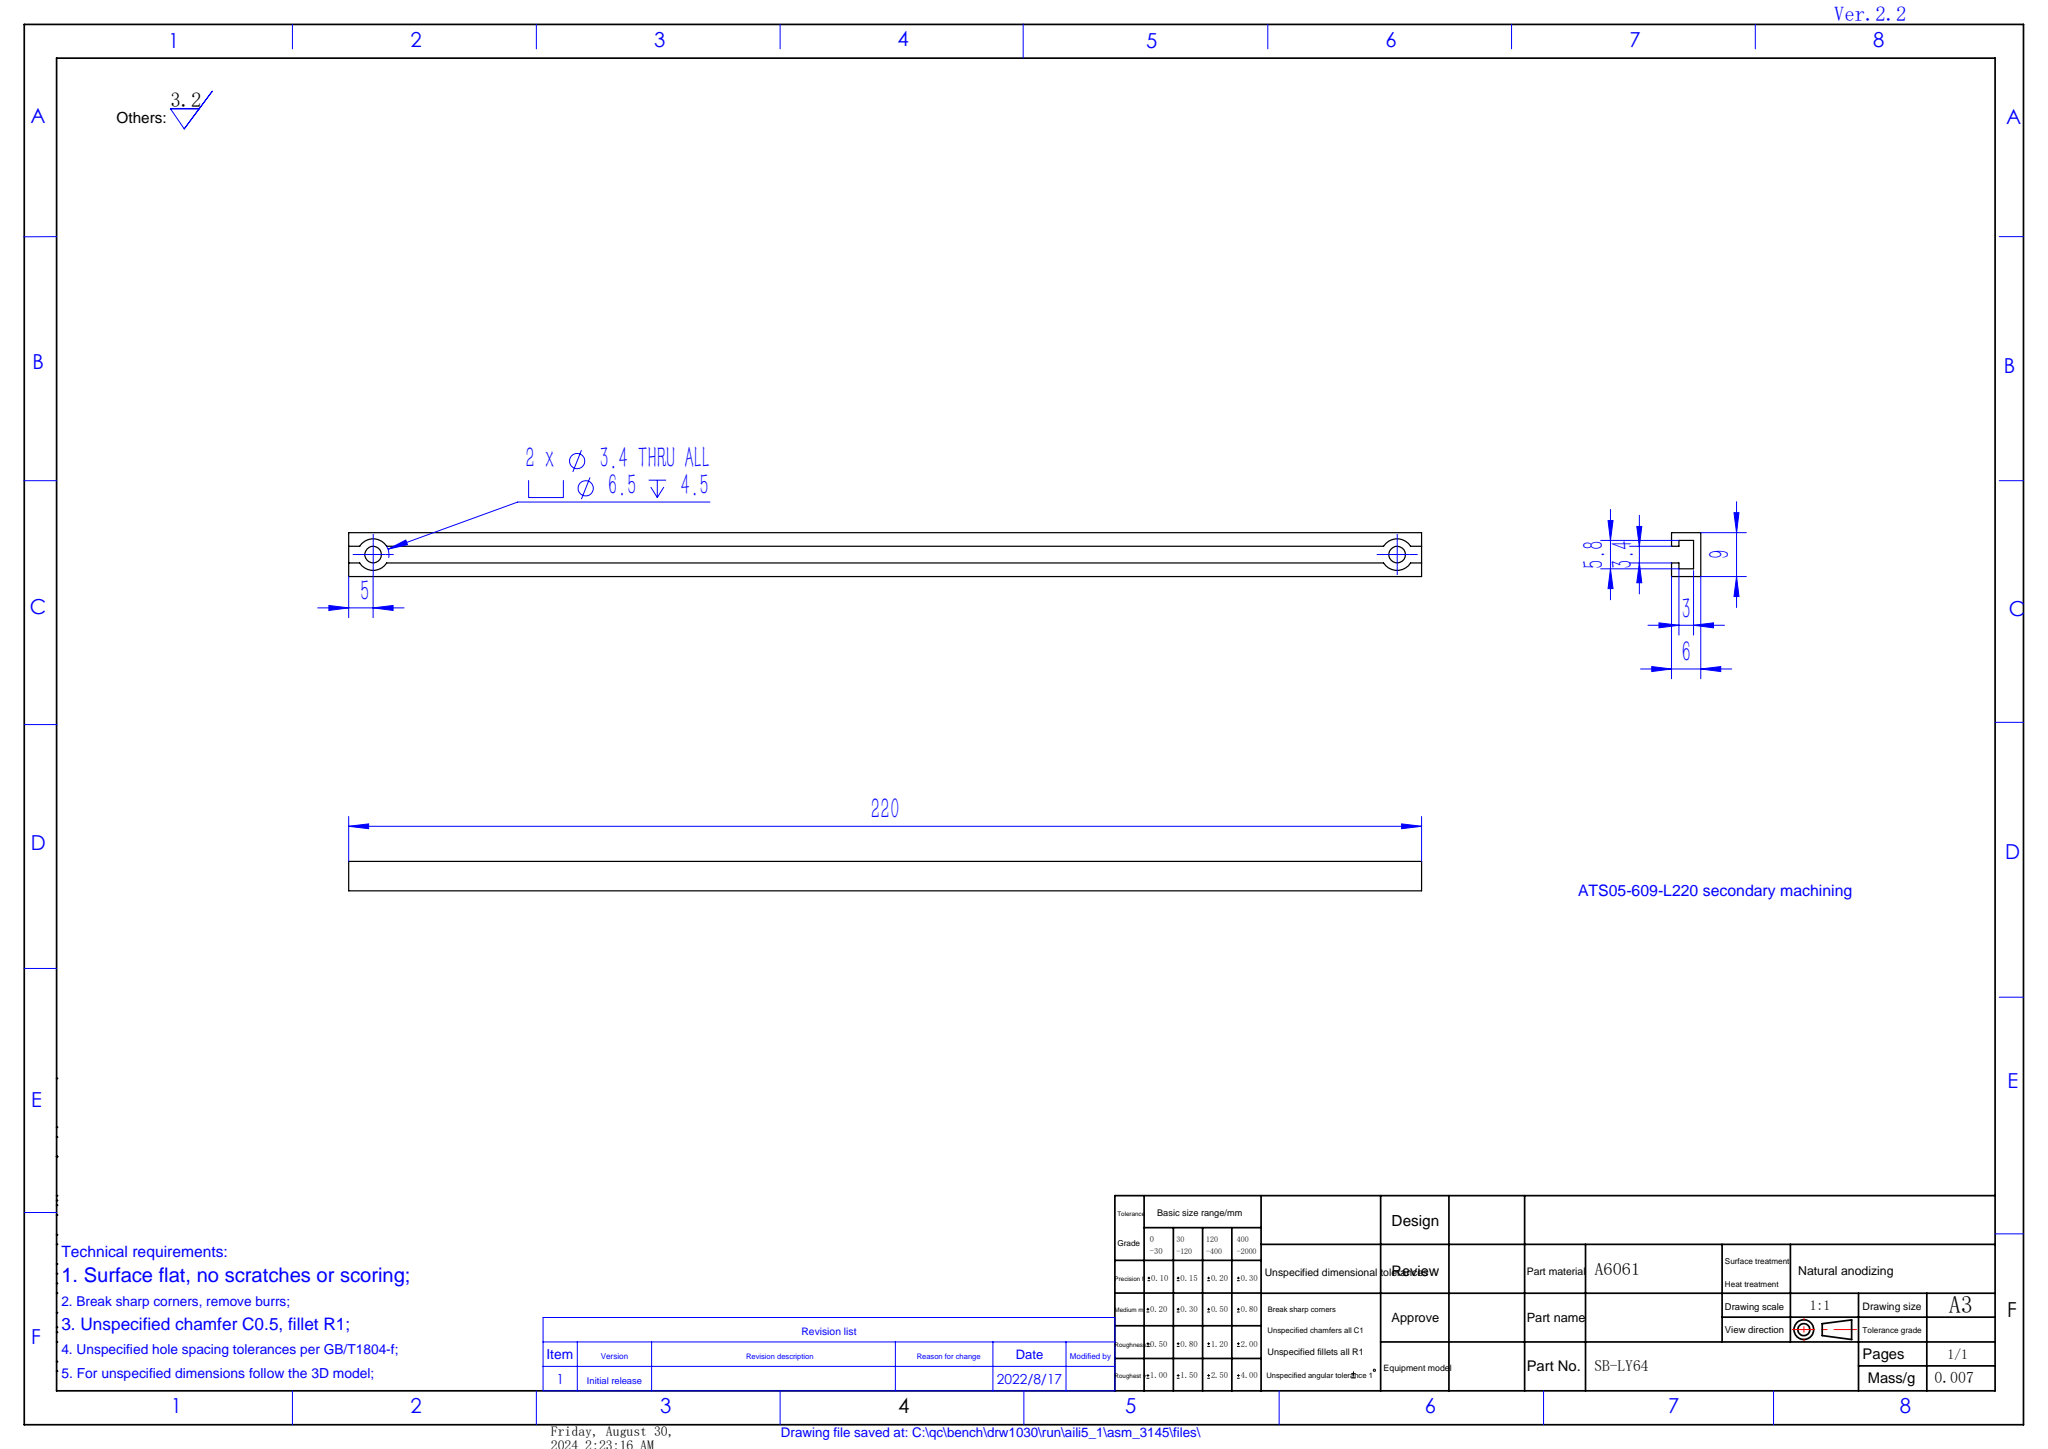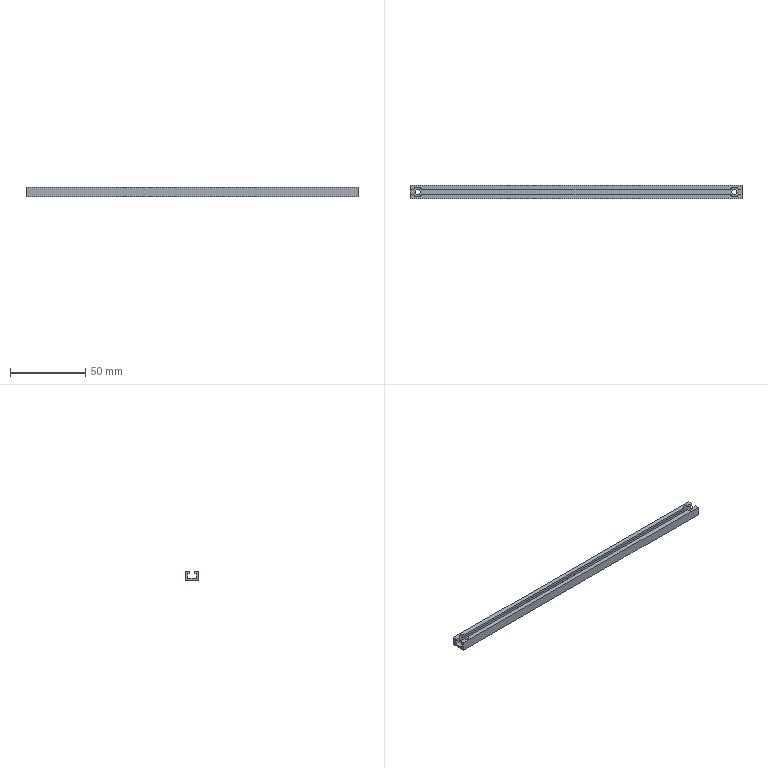Part | SolidWorks | features BaseBody 1, Cut 1, HoleWzd 1, ICE 1, MoveFace 1 | 1 solid | 34 faces | box 220 x 9 x 6 mm | volume 6858 mm3 | plane 26 | cylinder 8 | commonest cylinder face diameters 3.4 x4 6.5 x4